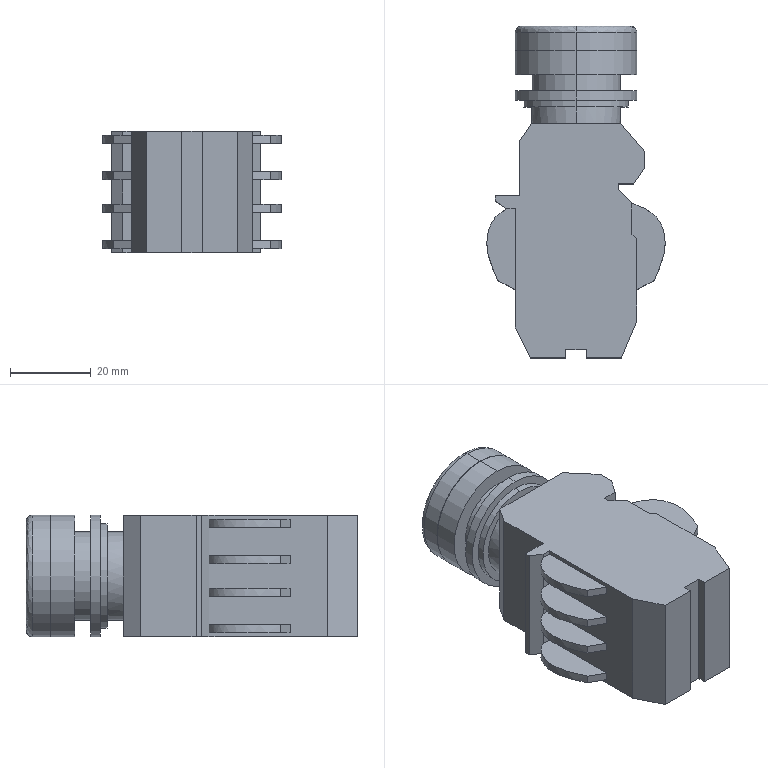Part | SolidWorks | features BaseBody 1 | 1 solid | 104 faces | box 44.081 x 82 x 30 mm | volume 65738 mm3 | plane 76 | cylinder 18 | spline 10 | commonest cylinder face diameters 30 x6 22 x4 25.7 x2 25.75 x2 25.901 x2 29.8 x2